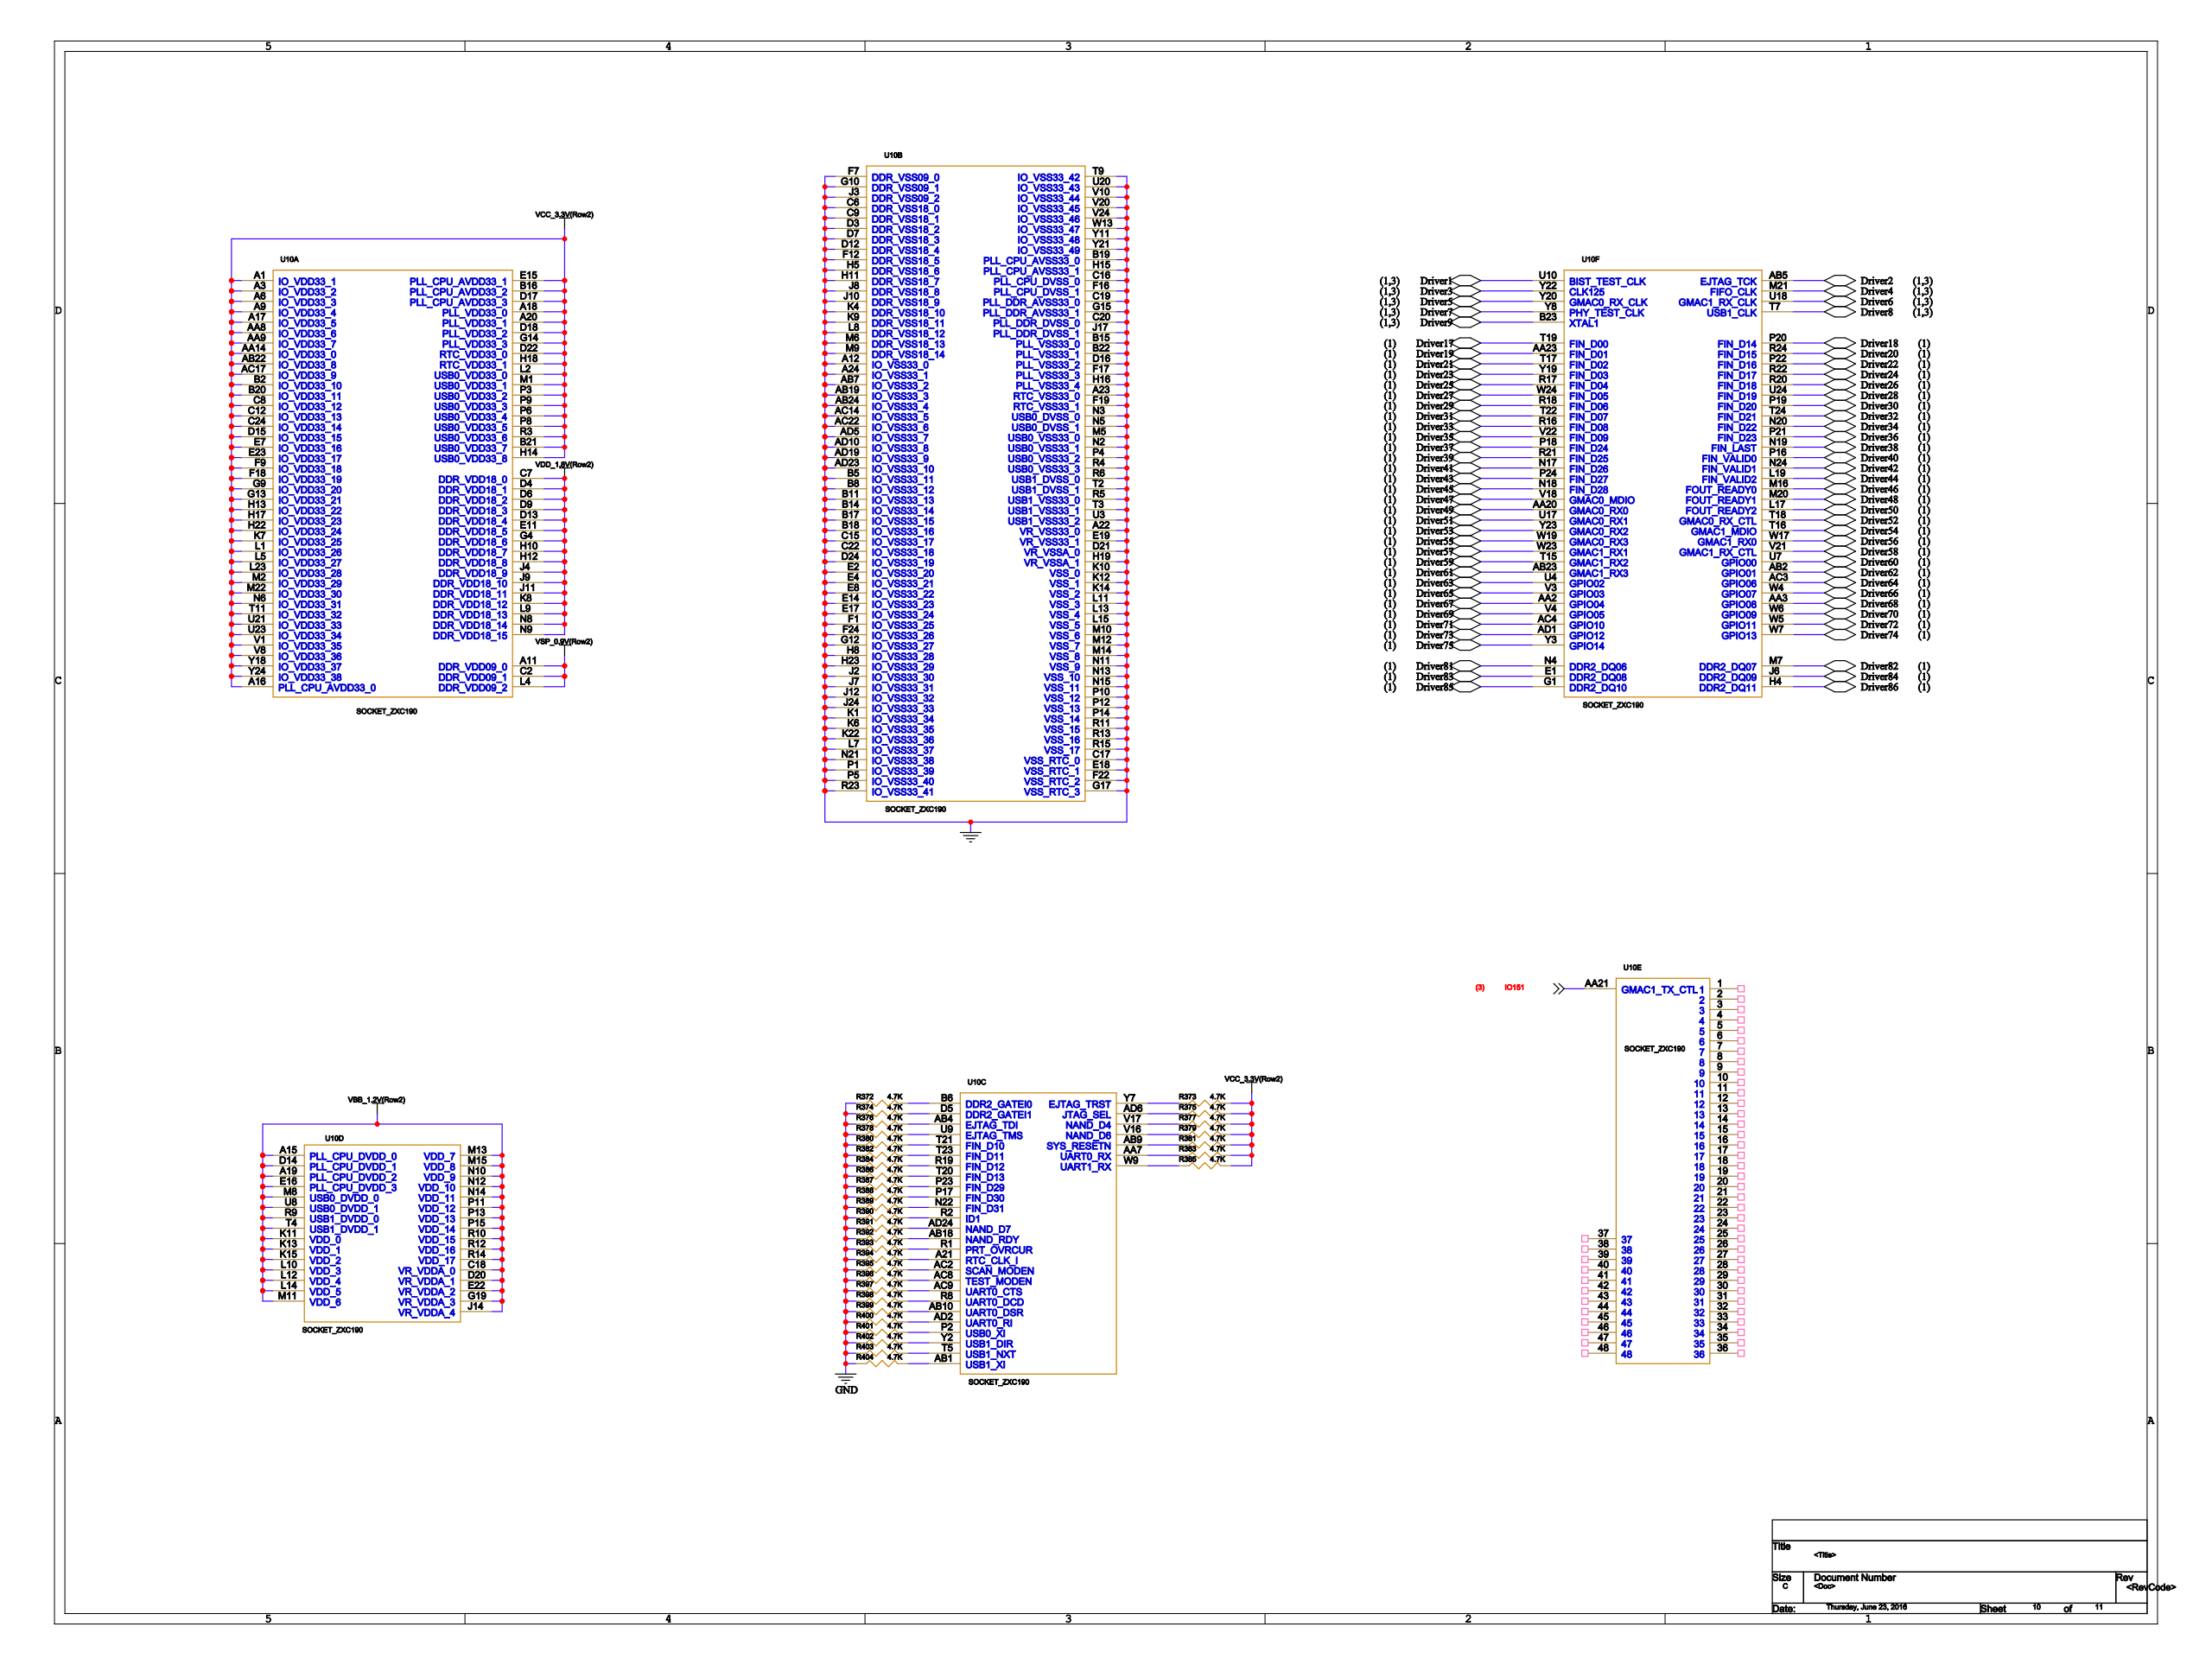Circuit board | Cadence Allegro | 531 parts | 624 nets | one sheet of the schematic
Parts on this sheet (reference | value | footprint):
R372 | 4.7K | R0805
R373 | 4.7K | R0805
R374 | 4.7K | R0805
R375 | 4.7K | R0805
R376 | 4.7K | R0805
R377 | 4.7K | R0805
R378 | 4.7K | R0805
R379 | 4.7K | R0805
R380 | 4.7K | R0805
R381 | 4.7K | R0805
R382 | 4.7K | R0805
R383 | 4.7K | R0805
R384 | 4.7K | R0805
R385 | 4.7K | R0805
R386 | 4.7K | R0805
R387 | 4.7K | R0805
R388 | 4.7K | R0805
R389 | 4.7K | R0805
R390 | 4.7K | R0805
R391 | 4.7K | R0805
R392 | 4.7K | R0805
R393 | 4.7K | R0805
R394 | 4.7K | R0805
R395 | 4.7K | R0805
R396 | 4.7K | R0805
R397 | 4.7K | R0805
R398 | 4.7K | R0805
R399 | 4.7K | R0805
R400 | 4.7K | R0805
R401 | 4.7K | R0805
R402 | 4.7K | R0805
R403 | 4.7K | R0805
R404 | 4.7K | R0805
U3 | SOCKET_ZXC190 | BGA-576
U4 | SOCKET_ZXC190 | BGA-576
U10 | SOCKET_ZXC190 | BGA-576
Nets of these parts (net: part-pin ...):
GND: R372-1 R374-1 R376-1 R378-1 R380-1 R382-1 R384-1 R386-1 R387-1 R388-1 R389-1 R390-1 R391-1 R392-1 R393-1 R394-1 R395-1 R396-1 R397-1 R398-1 R399-1 R400-1 R401-1 R402-1 R403-1 R404-1 U3-A12 U3-A22 U3-A23 U3-A24 U3-AB7 U3-AB19 U3-AB24 U3-AC14 U3-AC22 U3-AD5 U3-AD10 U3-AD19 U3-AD23 U3-B5 U3-B8 U3-B11 U3-B14 U3-B15 U3-B17 U3-B18 U3-B19 U3-B22 U3-C6 U3-C9 U3-C15 U3-C16 U3-C17 U3-C19 U3-C20 U3-C22 U3-D3 U3-D7 U3-D12 U3-D16 U3-D21 U3-D24 U3-E2 U3-E4 U3-E8 U3-E14 U3-E17 U3-E18 U3-E19 U3-F1 U3-F7 U3-F12 U3-F16 U3-F17 U3-F19 U3-F22 U3-F24 U3-G10 U3-G12 U3-G15 U3-G17 U3-H5 U3-H8 U3-H11 U3-H15 U3-H16 U3-H19 U3-H23 U3-J2 U3-J3 U3-J7 U3-J8 U3-J10 U3-J12 U3-J17 U3-J24 U3-K1 U3-K4 U3-K6 U3-K9 U3-K10 U3-K12 U3-K14 U3-K22 U3-L7 U3-L8 U3-L11 U3-L13 U3-L15 U3-M5 U3-M6 U3-M9 U3-M10 U3-M12 U3-M14 U3-N2 U3-N3 U3-N5 U3-N11 U3-N13 U3-N15 U3-N21 U3-P1 U3-P4 U3-P5 U3-P10 U3-P12 U3-P14 U3-R4 U3-R5 U3-R6 U3-R11 U3-R13 U3-R15 U3-R23 U3-T2 U3-T3 U3-T9 U3-U3 U3-U20 U3-V10 U3-V20 U3-V24 U3-W13 U3-Y11 U3-Y21 U4-A12 U4-A22 U4-A23 U4-A24 U4-AB7 U4-AB19 U4-AB24 U4-AC14 U4-AC22 U4-AD5 U4-AD10 U4-AD19 U4-AD23 U4-B5 U4-B8 U4-B11 U4-B14 U4-B15 U4-B17 U4-B18 U4-B19 U4-B22 U4-C6 U4-C9 U4-C15 U4-C16 U4-C17 U4-C19 U4-C20 U4-C22 U4-D3 U4-D7 U4-D12 U4-D16 U4-D21 U4-D24 U4-E2 U4-E4 U4-E8 U4-E14 U4-E17 U4-E18 U4-E19 U4-F1 U4-F7 U4-F12 U4-F16 U4-F17 U4-F19 U4-F22 U4-F24 U4-G10 U4-G12 U4-G15 U4-G17 U4-H5 U4-H8 U4-H11 U4-H15 U4-H16 U4-H19 U4-H23 U4-J2 U4-J3 U4-J7 U4-J8 U4-J10 U4-J12 U4-J17 U4-J24 U4-K1 U4-K4 U4-K6 U4-K9 U4-K10 U4-K12 U4-K14 U4-K22 U4-L7 U4-L8 U4-L11 U4-L13 U4-L15 U4-M5 U4-M6 U4-M9 U4-M10 U4-M12 U4-M14 U4-N2 U4-N3 U4-N5 U4-N11 U4-N13 U4-N15 U4-N21 U4-P1 U4-P4 U4-P5 U4-P10 U4-P12 U4-P14 U4-R4 U4-R5 U4-R6 U4-R11 U4-R13 U4-R15 U4-R23 U4-T2 U4-T3 U4-T9 U4-U3 U4-U20 U4-V10 U4-V20 U4-V24 U4-W13 U4-Y11 U4-Y21 U10-A12 U10-A22 U10-A23 U10-A24 U10-AB7 U10-AB19 U10-AB24 U10-AC14 U10-AC22 U10-AD5 U10-AD10 U10-AD19 U10-AD23 U10-B5 U10-B8 U10-B11 U10-B14 U10-B15 U10-B17 U10-B18 U10-B19 U10-B22 U10-C6 U10-C9 U10-C15 U10-C16 U10-C17 U10-C19 U10-C20 U10-C22 U10-D3 U10-D7 U10-D12 U10-D16 U10-D21 U10-D24 U10-E2 U10-E4 U10-E8 U10-E14 U10-E17 U10-E18 U10-E19 U10-F1 U10-F7 U10-F12 U10-F16 U10-F17 U10-F19 U10-F22 U10-F24 U10-G10 U10-G12 U10-G15 U10-G17 U10-H5 U10-H8 U10-H11 U10-H15 U10-H16 U10-H19 U10-H23 U10-J2 U10-J3 U10-J7 U10-J8 U10-J10 U10-J12 U10-J17 U10-J24 U10-K1 U10-K4 U10-K6 U10-K9 U10-K10 U10-K12 U10-K14 U10-K22 U10-L7 U10-L8 U10-L11 U10-L13 U10-L15 U10-M5 U10-M6 U10-M9 U10-M10 U10-M12 U10-M14 U10-N2 U10-N3 U10-N5 U10-N11 U10-N13 U10-N15 U10-N21 U10-P1 U10-P4 U10-P5 U10-P10 U10-P12 U10-P14 U10-R4 U10-R5 U10-R6 U10-R11 U10-R13 U10-R15 U10-R23 U10-T2 U10-T3 U10-T9 U10-U3 U10-U20 U10-V10 U10-V20 U10-V24 U10-W13 U10-Y11 U10-Y21
VCC_3.3V(ROW2): R373-2 R375-2 R377-2 R379-2 R381-2 R383-2 R385-2 U10-A1 U10-A3 U10-A6 U10-A9 U10-A16 U10-A17 U10-A18 U10-A20 U10-AA8 U10-AA9 U10-AA14 U10-AB22 U10-AC17 U10-B2 U10-B16 U10-B20 U10-B21 U10-C8 U10-C12 U10-C24 U10-D15 U10-D17 U10-D18 U10-D22 U10-E7 U10-E15 U10-E23 U10-F9 U10-F18 U10-G9 U10-G13 U10-G14 U10-H13 U10-H14 U10-H17 U10-H18 U10-H22 U10-K7 U10-L1 U10-L2 U10-L5 U10-L23 U10-M1 U10-M2 U10-M22 U10-N6 U10-P3 U10-P6 U10-P8 U10-P9 U10-R3 U10-T11 U10-U21 U10-U23 U10-V1 U10-V8 U10-Y18 U10-Y24
N8575690: R372-2 U10-B6
N8576098: R373-1 U10-Y7
N8575686: R374-2 U10-D5
N8576134: R375-1 U10-AD6
N8575682: R376-2 U10-AB4
N8576294: R377-1 U10-V17
N8575678: R378-2 U10-U9
N8576298: R379-1 U10-V16
N8575674: R380-2 U10-T21
N8576306: R381-1 U10-AB9
N8575654: R382-2 U10-T23
N8576302: R383-1 U10-AA7
N8575650: R384-2 U10-R19
N8575646: R385-1 U10-W9
N8575722: R386-2 U10-T20
N8575718: R387-2 U10-P23
N8575714: R388-2 U10-P17
N8575710: R389-2 U10-N22
N8575706: R390-2 U10-R2
N8575702: R391-2 U10-AD24
N8575698: R392-2 U10-AB18
N8575694: R393-2 U10-R1
N8575750: R394-2 U10-A21
N8575746: R395-2 U10-AC2
N8575742: R396-2 U10-AC8
N8575738: R397-2 U10-AC9
N8576186: R398-2 U10-R8
N8575734: R399-2 U10-AB10
N8575730: R400-2 U10-AD2
N8575726: R401-2 U10-P2
N8575762: R402-2 U10-Y2
N8575758: R403-2 U10-T5
N8575754: R404-2 U10-AB1
IO151: U10-AA21